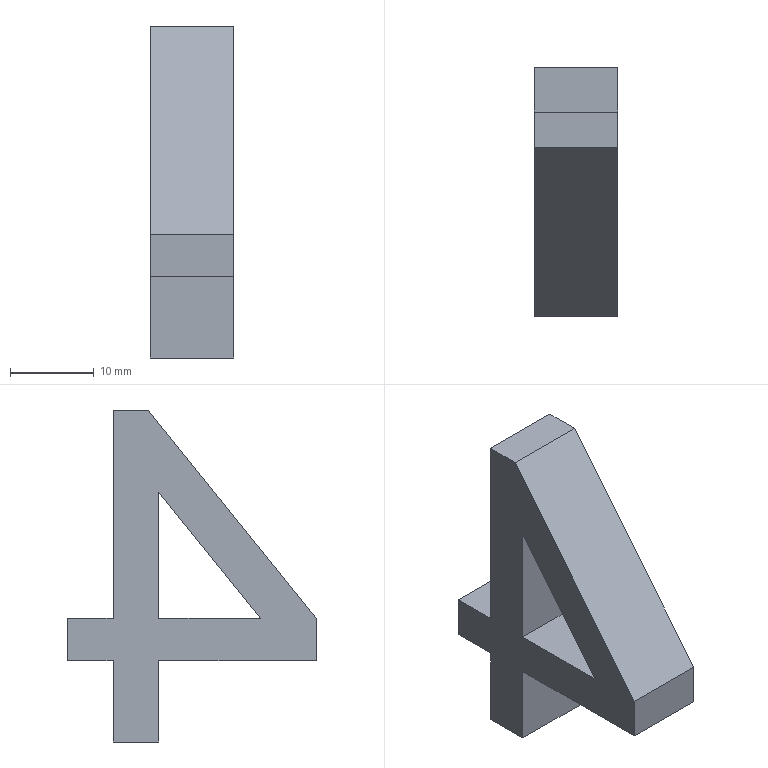Part | NX | features solid 2 | 1 solid | 16 faces | box 10 x 29.69 x 39.602 mm | volume 4649 mm3 | plane 16
STEP:
#1=CARTESIAN_POINT('',(2250.,-423.385,-655.254));
#2=VERTEX_POINT('',#1);
#3=CARTESIAN_POINT('',(2250.,-423.385,-640.218));
#4=VERTEX_POINT('',#3);
#5=CARTESIAN_POINT('',(2250.,-423.385,-655.254));
#6=CARTESIAN_POINT('',(2250.,-423.385,-650.242));
#7=CARTESIAN_POINT('',(2250.,-423.385,-645.23));
#8=CARTESIAN_POINT('',(2250.,-423.385,-640.218));
#9=B_SPLINE_CURVE_WITH_KNOTS('',3,(#5,#6,#7,#8),.UNSPECIFIED.,.F.,.F.,(4,4),(0.2613,0.5844),.PIECEWISE_BEZIER_KNOTS.);
#10=EDGE_CURVE('',#2,#4,#9,.T.);
#11=ORIENTED_EDGE('',*,*,#10,.F.);
#12=CARTESIAN_POINT('',(2260.,-423.385,-655.254));
#13=VERTEX_POINT('',#12);
#14=CARTESIAN_POINT('',(2260.,-423.385,-655.254));
#15=DIRECTION('',(-1.,0.,0.));
#16=VECTOR('',#15,1000.);
#17=LINE('',#14,#16);
#18=EDGE_CURVE('',#13,#2,#17,.T.);
#19=ORIENTED_EDGE('',*,*,#18,.F.);
#20=CARTESIAN_POINT('',(2260.,-423.385,-640.218));
#21=VERTEX_POINT('',#20);
#22=CARTESIAN_POINT('',(2260.,-423.385,-655.254));
#23=CARTESIAN_POINT('',(2260.,-423.385,-650.242));
#24=CARTESIAN_POINT('',(2260.,-423.385,-645.23));
#25=CARTESIAN_POINT('',(2260.,-423.385,-640.218));
#26=B_SPLINE_CURVE_WITH_KNOTS('',3,(#22,#23,#24,#25),.UNSPECIFIED.,.F.,.F.,(4,4),(0.2613,0.5844),.PIECEWISE_BEZIER_KNOTS.);
#27=EDGE_CURVE('',#13,#21,#26,.T.);
#28=ORIENTED_EDGE('',*,*,#27,.T.);
#29=CARTESIAN_POINT('',(2260.,-423.385,-640.218));
#30=DIRECTION('',(-1.,0.,0.));
#31=VECTOR('',#30,1000.);
#32=LINE('',#29,#31);
#33=EDGE_CURVE('',#21,#4,#32,.T.);
#34=ORIENTED_EDGE('',*,*,#33,.T.);
#35=EDGE_LOOP('',(#11,#19,#28,#34));
#36=FACE_BOUND('',#35,.T.);
#37=CARTESIAN_POINT('',(2260.,-423.385,-655.254));
#38=DIRECTION('',(0.,-1.,0.));
#39=DIRECTION('',(1.,0.,0.));
#40=AXIS2_PLACEMENT_3D('',#37,#38,#39);
#41=PLANE('',#40);
#42=ADVANCED_FACE('',(#36),#41,.T.);
#43=CARTESIAN_POINT('',(2250.,-435.546,-655.254));
#44=VERTEX_POINT('',#43);
#45=CARTESIAN_POINT('',(2250.,-423.385,-640.218));
#46=CARTESIAN_POINT('',(2250.,-427.439,-645.23));
#47=CARTESIAN_POINT('',(2250.,-431.493,-650.242));
#48=CARTESIAN_POINT('',(2250.,-435.546,-655.254));
#49=B_SPLINE_CURVE_WITH_KNOTS('',3,(#45,#46,#47,#48),.UNSPECIFIED.,.F.,.F.,(4,4),(0.5844,1.),.PIECEWISE_BEZIER_KNOTS.);
#50=EDGE_CURVE('',#4,#44,#49,.T.);
#51=ORIENTED_EDGE('',*,*,#50,.F.);
#52=ORIENTED_EDGE('',*,*,#33,.F.);
#53=CARTESIAN_POINT('',(2260.,-435.546,-655.254));
#54=VERTEX_POINT('',#53);
#55=CARTESIAN_POINT('',(2260.,-423.385,-640.218));
#56=CARTESIAN_POINT('',(2260.,-427.439,-645.23));
#57=CARTESIAN_POINT('',(2260.,-431.493,-650.242));
#58=CARTESIAN_POINT('',(2260.,-435.546,-655.254));
#59=B_SPLINE_CURVE_WITH_KNOTS('',3,(#55,#56,#57,#58),.UNSPECIFIED.,.F.,.F.,(4,4),(0.5844,1.),.PIECEWISE_BEZIER_KNOTS.);
#60=EDGE_CURVE('',#21,#54,#59,.T.);
#61=ORIENTED_EDGE('',*,*,#60,.T.);
#62=CARTESIAN_POINT('',(2260.,-435.546,-655.254));
#63=DIRECTION('',(-1.,0.,0.));
#64=VECTOR('',#63,1000.);
#65=LINE('',#62,#64);
#66=EDGE_CURVE('',#54,#44,#65,.T.);
#67=ORIENTED_EDGE('',*,*,#66,.T.);
#68=EDGE_LOOP('',(#51,#52,#61,#67));
#69=FACE_BOUND('',#68,.T.);
#70=CARTESIAN_POINT('',(2260.,-423.385,-640.218));
#71=DIRECTION('',(0.,0.7775,-0.6288));
#72=DIRECTION('',(0.,0.6288,0.7775));
#73=AXIS2_PLACEMENT_3D('',#70,#71,#72);
#74=PLANE('',#73);
#75=ADVANCED_FACE('',(#69),#74,.T.);
#76=CARTESIAN_POINT('',(2250.,-417.94,-670.));
#77=VERTEX_POINT('',#76);
#78=CARTESIAN_POINT('',(2250.,-423.385,-670.));
#79=VERTEX_POINT('',#78);
#80=CARTESIAN_POINT('',(2250.,-417.94,-670.));
#81=CARTESIAN_POINT('',(2250.,-419.755,-670.));
#82=CARTESIAN_POINT('',(2250.,-421.57,-670.));
#83=CARTESIAN_POINT('',(2250.,-423.385,-670.));
#84=B_SPLINE_CURVE_WITH_KNOTS('',3,(#80,#81,#82,#83),.UNSPECIFIED.,.F.,.F.,(4,4),(0.,0.04335),.PIECEWISE_BEZIER_KNOTS.);
#85=EDGE_CURVE('',#77,#79,#84,.T.);
#86=ORIENTED_EDGE('',*,*,#85,.F.);
#87=CARTESIAN_POINT('',(2260.,-417.94,-670.));
#88=VERTEX_POINT('',#87);
#89=CARTESIAN_POINT('',(2260.,-417.94,-670.));
#90=DIRECTION('',(-1.,0.,0.));
#91=VECTOR('',#90,1000.);
#92=LINE('',#89,#91);
#93=EDGE_CURVE('',#88,#77,#92,.T.);
#94=ORIENTED_EDGE('',*,*,#93,.F.);
#95=CARTESIAN_POINT('',(2260.,-423.385,-670.));
#96=VERTEX_POINT('',#95);
#97=CARTESIAN_POINT('',(2260.,-417.94,-670.));
#98=CARTESIAN_POINT('',(2260.,-419.755,-670.));
#99=CARTESIAN_POINT('',(2260.,-421.57,-670.));
#100=CARTESIAN_POINT('',(2260.,-423.385,-670.));
#101=B_SPLINE_CURVE_WITH_KNOTS('',3,(#97,#98,#99,#100),.UNSPECIFIED.,.F.,.F.,(4,4),(0.,0.04335),.PIECEWISE_BEZIER_KNOTS.);
#102=EDGE_CURVE('',#88,#96,#101,.T.);
#103=ORIENTED_EDGE('',*,*,#102,.T.);
#104=CARTESIAN_POINT('',(2260.,-423.385,-670.));
#105=DIRECTION('',(-1.,0.,0.));
#106=VECTOR('',#105,1000.);
#107=LINE('',#104,#106);
#108=EDGE_CURVE('',#96,#79,#107,.T.);
#109=ORIENTED_EDGE('',*,*,#108,.T.);
#110=EDGE_LOOP('',(#86,#94,#103,#109));
#111=FACE_BOUND('',#110,.T.);
#112=CARTESIAN_POINT('',(2260.,-417.94,-670.));
#113=DIRECTION('',(0.,0.,-1.));
#114=DIRECTION('',(-1.,0.,0.));
#115=AXIS2_PLACEMENT_3D('',#112,#113,#114);
#116=PLANE('',#115);
#117=ADVANCED_FACE('',(#111),#116,.T.);
#118=CARTESIAN_POINT('',(2250.,-423.385,-660.302));
#119=VERTEX_POINT('',#118);
#120=CARTESIAN_POINT('',(2250.,-423.385,-670.));
#121=CARTESIAN_POINT('',(2250.,-423.385,-666.767));
#122=CARTESIAN_POINT('',(2250.,-423.385,-663.535));
#123=CARTESIAN_POINT('',(2250.,-423.385,-660.302));
#124=B_SPLINE_CURVE_WITH_KNOTS('',3,(#120,#121,#122,#123),.UNSPECIFIED.,.F.,.F.,(4,4),(0.04335,0.1206),.PIECEWISE_BEZIER_KNOTS.);
#125=EDGE_CURVE('',#79,#119,#124,.T.);
#126=ORIENTED_EDGE('',*,*,#125,.F.);
#127=ORIENTED_EDGE('',*,*,#108,.F.);
#128=CARTESIAN_POINT('',(2260.,-423.385,-660.302));
#129=VERTEX_POINT('',#128);
#130=CARTESIAN_POINT('',(2260.,-423.385,-670.));
#131=CARTESIAN_POINT('',(2260.,-423.385,-666.767));
#132=CARTESIAN_POINT('',(2260.,-423.385,-663.535));
#133=CARTESIAN_POINT('',(2260.,-423.385,-660.302));
#134=B_SPLINE_CURVE_WITH_KNOTS('',3,(#130,#131,#132,#133),.UNSPECIFIED.,.F.,.F.,(4,4),(0.04335,0.1206),.PIECEWISE_BEZIER_KNOTS.);
#135=EDGE_CURVE('',#96,#129,#134,.T.);
#136=ORIENTED_EDGE('',*,*,#135,.T.);
#137=CARTESIAN_POINT('',(2260.,-423.385,-660.302));
#138=DIRECTION('',(-1.,0.,0.));
#139=VECTOR('',#138,1000.);
#140=LINE('',#137,#139);
#141=EDGE_CURVE('',#129,#119,#140,.T.);
#142=ORIENTED_EDGE('',*,*,#141,.T.);
#143=EDGE_LOOP('',(#126,#127,#136,#142));
#144=FACE_BOUND('',#143,.T.);
#145=CARTESIAN_POINT('',(2260.,-423.385,-670.));
#146=DIRECTION('',(0.,-1.,0.));
#147=DIRECTION('',(1.,0.,0.));
#148=AXIS2_PLACEMENT_3D('',#145,#146,#147);
#149=PLANE('',#148);
#150=ADVANCED_FACE('',(#144),#149,.T.);
#151=CARTESIAN_POINT('',(2250.,-442.2,-660.302));
#152=VERTEX_POINT('',#151);
#153=CARTESIAN_POINT('',(2250.,-423.385,-660.302));
#154=CARTESIAN_POINT('',(2250.,-429.657,-660.302));
#155=CARTESIAN_POINT('',(2250.,-435.928,-660.302));
#156=CARTESIAN_POINT('',(2250.,-442.2,-660.302));
#157=B_SPLINE_CURVE_WITH_KNOTS('',3,(#153,#154,#155,#156),.UNSPECIFIED.,.F.,.F.,(4,4),(0.1206,0.2704),.PIECEWISE_BEZIER_KNOTS.);
#158=EDGE_CURVE('',#119,#152,#157,.T.);
#159=ORIENTED_EDGE('',*,*,#158,.F.);
#160=ORIENTED_EDGE('',*,*,#141,.F.);
#161=CARTESIAN_POINT('',(2260.,-442.2,-660.302));
#162=VERTEX_POINT('',#161);
#163=CARTESIAN_POINT('',(2260.,-423.385,-660.302));
#164=CARTESIAN_POINT('',(2260.,-429.657,-660.302));
#165=CARTESIAN_POINT('',(2260.,-435.928,-660.302));
#166=CARTESIAN_POINT('',(2260.,-442.2,-660.302));
#167=B_SPLINE_CURVE_WITH_KNOTS('',3,(#163,#164,#165,#166),.UNSPECIFIED.,.F.,.F.,(4,4),(0.1206,0.2704),.PIECEWISE_BEZIER_KNOTS.);
#168=EDGE_CURVE('',#129,#162,#167,.T.);
#169=ORIENTED_EDGE('',*,*,#168,.T.);
#170=CARTESIAN_POINT('',(2260.,-442.2,-660.302));
#171=DIRECTION('',(-1.,0.,0.));
#172=VECTOR('',#171,1000.);
#173=LINE('',#170,#172);
#174=EDGE_CURVE('',#162,#152,#173,.T.);
#175=ORIENTED_EDGE('',*,*,#174,.T.);
#176=EDGE_LOOP('',(#159,#160,#169,#175));
#177=FACE_BOUND('',#176,.T.);
#178=CARTESIAN_POINT('',(2260.,-423.385,-660.302));
#179=DIRECTION('',(0.,0.,-1.));
#180=DIRECTION('',(-1.,0.,0.));
#181=AXIS2_PLACEMENT_3D('',#178,#179,#180);
#182=PLANE('',#181);
#183=ADVANCED_FACE('',(#177),#182,.T.);
#184=CARTESIAN_POINT('',(2250.,-442.2,-655.254));
#185=VERTEX_POINT('',#184);
#186=CARTESIAN_POINT('',(2250.,-442.2,-660.302));
#187=CARTESIAN_POINT('',(2250.,-442.2,-658.62));
#188=CARTESIAN_POINT('',(2250.,-442.2,-656.937));
#189=CARTESIAN_POINT('',(2250.,-442.2,-655.254));
#190=B_SPLINE_CURVE_WITH_KNOTS('',3,(#186,#187,#188,#189),.UNSPECIFIED.,.F.,.F.,(4,4),(0.2704,0.3105),.PIECEWISE_BEZIER_KNOTS.);
#191=EDGE_CURVE('',#152,#185,#190,.T.);
#192=ORIENTED_EDGE('',*,*,#191,.F.);
#193=ORIENTED_EDGE('',*,*,#174,.F.);
#194=CARTESIAN_POINT('',(2260.,-442.2,-655.254));
#195=VERTEX_POINT('',#194);
#196=CARTESIAN_POINT('',(2260.,-442.2,-660.302));
#197=CARTESIAN_POINT('',(2260.,-442.2,-658.62));
#198=CARTESIAN_POINT('',(2260.,-442.2,-656.937));
#199=CARTESIAN_POINT('',(2260.,-442.2,-655.254));
#200=B_SPLINE_CURVE_WITH_KNOTS('',3,(#196,#197,#198,#199),.UNSPECIFIED.,.F.,.F.,(4,4),(0.2704,0.3105),.PIECEWISE_BEZIER_KNOTS.);
#201=EDGE_CURVE('',#162,#195,#200,.T.);
#202=ORIENTED_EDGE('',*,*,#201,.T.);
#203=CARTESIAN_POINT('',(2260.,-442.2,-655.254));
#204=DIRECTION('',(-1.,0.,0.));
#205=VECTOR('',#204,1000.);
#206=LINE('',#203,#205);
#207=EDGE_CURVE('',#195,#185,#206,.T.);
#208=ORIENTED_EDGE('',*,*,#207,.T.);
#209=EDGE_LOOP('',(#192,#193,#202,#208));
#210=FACE_BOUND('',#209,.T.);
#211=CARTESIAN_POINT('',(2260.,-442.2,-660.302));
#212=DIRECTION('',(0.,-1.,0.));
#213=DIRECTION('',(1.,0.,0.));
#214=AXIS2_PLACEMENT_3D('',#211,#212,#213);
#215=PLANE('',#214);
#216=ADVANCED_FACE('',(#210),#215,.T.);
#217=CARTESIAN_POINT('',(2250.,-422.131,-630.398));
#218=VERTEX_POINT('',#217);
#219=CARTESIAN_POINT('',(2250.,-442.2,-655.254));
#220=CARTESIAN_POINT('',(2250.,-435.51,-646.969));
#221=CARTESIAN_POINT('',(2250.,-428.821,-638.683));
#222=CARTESIAN_POINT('',(2250.,-422.131,-630.398));
#223=B_SPLINE_CURVE_WITH_KNOTS('',3,(#219,#220,#221,#222),.UNSPECIFIED.,.F.,.F.,(4,4),(0.3105,0.5649),.PIECEWISE_BEZIER_KNOTS.);
#224=EDGE_CURVE('',#185,#218,#223,.T.);
#225=ORIENTED_EDGE('',*,*,#224,.F.);
#226=ORIENTED_EDGE('',*,*,#207,.F.);
#227=CARTESIAN_POINT('',(2260.,-422.131,-630.398));
#228=VERTEX_POINT('',#227);
#229=CARTESIAN_POINT('',(2260.,-442.2,-655.254));
#230=CARTESIAN_POINT('',(2260.,-435.51,-646.969));
#231=CARTESIAN_POINT('',(2260.,-428.821,-638.683));
#232=CARTESIAN_POINT('',(2260.,-422.131,-630.398));
#233=B_SPLINE_CURVE_WITH_KNOTS('',3,(#229,#230,#231,#232),.UNSPECIFIED.,.F.,.F.,(4,4),(0.3105,0.5649),.PIECEWISE_BEZIER_KNOTS.);
#234=EDGE_CURVE('',#195,#228,#233,.T.);
#235=ORIENTED_EDGE('',*,*,#234,.T.);
#236=CARTESIAN_POINT('',(2260.,-422.131,-630.398));
#237=DIRECTION('',(-1.,0.,0.));
#238=VECTOR('',#237,1000.);
#239=LINE('',#236,#238);
#240=EDGE_CURVE('',#228,#218,#239,.T.);
#241=ORIENTED_EDGE('',*,*,#240,.T.);
#242=EDGE_LOOP('',(#225,#226,#235,#241));
#243=FACE_BOUND('',#242,.T.);
#244=CARTESIAN_POINT('',(2260.,-442.2,-655.254));
#245=DIRECTION('',(0.,-0.7781,0.6282));
#246=DIRECTION('',(0.,-0.6282,-0.7781));
#247=AXIS2_PLACEMENT_3D('',#244,#245,#246);
#248=PLANE('',#247);
#249=ADVANCED_FACE('',(#243),#248,.T.);
#250=CARTESIAN_POINT('',(2250.,-417.94,-630.398));
#251=VERTEX_POINT('',#250);
#252=CARTESIAN_POINT('',(2250.,-422.131,-630.398));
#253=CARTESIAN_POINT('',(2250.,-420.734,-630.398));
#254=CARTESIAN_POINT('',(2250.,-419.337,-630.398));
#255=CARTESIAN_POINT('',(2250.,-417.94,-630.398));
#256=B_SPLINE_CURVE_WITH_KNOTS('',3,(#252,#253,#254,#255),.UNSPECIFIED.,.F.,.F.,(4,4),(0.5649,0.5982),.PIECEWISE_BEZIER_KNOTS.);
#257=EDGE_CURVE('',#218,#251,#256,.T.);
#258=ORIENTED_EDGE('',*,*,#257,.F.);
#259=ORIENTED_EDGE('',*,*,#240,.F.);
#260=CARTESIAN_POINT('',(2260.,-417.94,-630.398));
#261=VERTEX_POINT('',#260);
#262=CARTESIAN_POINT('',(2260.,-422.131,-630.398));
#263=CARTESIAN_POINT('',(2260.,-420.734,-630.398));
#264=CARTESIAN_POINT('',(2260.,-419.337,-630.398));
#265=CARTESIAN_POINT('',(2260.,-417.94,-630.398));
#266=B_SPLINE_CURVE_WITH_KNOTS('',3,(#262,#263,#264,#265),.UNSPECIFIED.,.F.,.F.,(4,4),(0.5649,0.5982),.PIECEWISE_BEZIER_KNOTS.);
#267=EDGE_CURVE('',#228,#261,#266,.T.);
#268=ORIENTED_EDGE('',*,*,#267,.T.);
#269=CARTESIAN_POINT('',(2260.,-417.94,-630.398));
#270=DIRECTION('',(-1.,0.,0.));
#271=VECTOR('',#270,1000.);
#272=LINE('',#269,#271);
#273=EDGE_CURVE('',#261,#251,#272,.T.);
#274=ORIENTED_EDGE('',*,*,#273,.T.);
#275=EDGE_LOOP('',(#258,#259,#268,#274));
#276=FACE_BOUND('',#275,.T.);
#277=CARTESIAN_POINT('',(2260.,-422.131,-630.398));
#278=DIRECTION('',(0.,0.,1.));
#279=DIRECTION('',(1.,0.,0.));
#280=AXIS2_PLACEMENT_3D('',#277,#278,#279);
#281=PLANE('',#280);
#282=ADVANCED_FACE('',(#276),#281,.T.);
#283=CARTESIAN_POINT('',(2250.,-417.94,-655.254));
#284=VERTEX_POINT('',#283);
#285=CARTESIAN_POINT('',(2250.,-417.94,-630.398));
#286=CARTESIAN_POINT('',(2250.,-417.94,-638.683));
#287=CARTESIAN_POINT('',(2250.,-417.94,-646.969));
#288=CARTESIAN_POINT('',(2250.,-417.94,-655.254));
#289=B_SPLINE_CURVE_WITH_KNOTS('',3,(#285,#286,#287,#288),.UNSPECIFIED.,.F.,.F.,(4,4),(0.5982,0.7961),.PIECEWISE_BEZIER_KNOTS.);
#290=EDGE_CURVE('',#251,#284,#289,.T.);
#291=ORIENTED_EDGE('',*,*,#290,.F.);
#292=ORIENTED_EDGE('',*,*,#273,.F.);
#293=CARTESIAN_POINT('',(2260.,-417.94,-655.254));
#294=VERTEX_POINT('',#293);
#295=CARTESIAN_POINT('',(2260.,-417.94,-630.398));
#296=CARTESIAN_POINT('',(2260.,-417.94,-638.683));
#297=CARTESIAN_POINT('',(2260.,-417.94,-646.969));
#298=CARTESIAN_POINT('',(2260.,-417.94,-655.254));
#299=B_SPLINE_CURVE_WITH_KNOTS('',3,(#295,#296,#297,#298),.UNSPECIFIED.,.F.,.F.,(4,4),(0.5982,0.7961),.PIECEWISE_BEZIER_KNOTS.);
#300=EDGE_CURVE('',#261,#294,#299,.T.);
#301=ORIENTED_EDGE('',*,*,#300,.T.);
#302=CARTESIAN_POINT('',(2260.,-417.94,-655.254));
#303=DIRECTION('',(-1.,0.,0.));
#304=VECTOR('',#303,1000.);
#305=LINE('',#302,#304);
#306=EDGE_CURVE('',#294,#284,#305,.T.);
#307=ORIENTED_EDGE('',*,*,#306,.T.);
#308=EDGE_LOOP('',(#291,#292,#301,#307));
#309=FACE_BOUND('',#308,.T.);
#310=CARTESIAN_POINT('',(2260.,-417.94,-630.398));
#311=DIRECTION('',(0.,1.,0.));
#312=DIRECTION('',(-1.,0.,0.));
#313=AXIS2_PLACEMENT_3D('',#310,#311,#312);
#314=PLANE('',#313);
#315=ADVANCED_FACE('',(#309),#314,.T.);
#316=CARTESIAN_POINT('',(2250.,-412.51,-655.254));
#317=VERTEX_POINT('',#316);
#318=CARTESIAN_POINT('',(2250.,-417.94,-655.254));
#319=CARTESIAN_POINT('',(2250.,-416.13,-655.254));
#320=CARTESIAN_POINT('',(2250.,-414.32,-655.254));
#321=CARTESIAN_POINT('',(2250.,-412.51,-655.254));
#322=B_SPLINE_CURVE_WITH_KNOTS('',3,(#318,#319,#320,#321),.UNSPECIFIED.,.F.,.F.,(4,4),(0.7961,0.8394),.PIECEWISE_BEZIER_KNOTS.);
#323=EDGE_CURVE('',#284,#317,#322,.T.);
#324=ORIENTED_EDGE('',*,*,#323,.F.);
#325=ORIENTED_EDGE('',*,*,#306,.F.);
#326=CARTESIAN_POINT('',(2260.,-412.51,-655.254));
#327=VERTEX_POINT('',#326);
#328=CARTESIAN_POINT('',(2260.,-417.94,-655.254));
#329=CARTESIAN_POINT('',(2260.,-416.13,-655.254));
#330=CARTESIAN_POINT('',(2260.,-414.32,-655.254));
#331=CARTESIAN_POINT('',(2260.,-412.51,-655.254));
#332=B_SPLINE_CURVE_WITH_KNOTS('',3,(#328,#329,#330,#331),.UNSPECIFIED.,.F.,.F.,(4,4),(0.7961,0.8394),.PIECEWISE_BEZIER_KNOTS.);
#333=EDGE_CURVE('',#294,#327,#332,.T.);
#334=ORIENTED_EDGE('',*,*,#333,.T.);
#335=CARTESIAN_POINT('',(2260.,-412.51,-655.254));
#336=DIRECTION('',(-1.,0.,0.));
#337=VECTOR('',#336,1000.);
#338=LINE('',#335,#337);
#339=EDGE_CURVE('',#327,#317,#338,.T.);
#340=ORIENTED_EDGE('',*,*,#339,.T.);
#341=EDGE_LOOP('',(#324,#325,#334,#340));
#342=FACE_BOUND('',#341,.T.);
#343=CARTESIAN_POINT('',(2260.,-417.94,-655.254));
#344=DIRECTION('',(0.,0.,1.));
#345=DIRECTION('',(1.,0.,0.));
#346=AXIS2_PLACEMENT_3D('',#343,#344,#345);
#347=PLANE('',#346);
#348=ADVANCED_FACE('',(#342),#347,.T.);
#349=CARTESIAN_POINT('',(2250.,-412.51,-660.302));
#350=VERTEX_POINT('',#349);
#351=CARTESIAN_POINT('',(2250.,-412.51,-655.254));
#352=CARTESIAN_POINT('',(2250.,-412.51,-656.937));
#353=CARTESIAN_POINT('',(2250.,-412.51,-658.62));
#354=CARTESIAN_POINT('',(2250.,-412.51,-660.302));
#355=B_SPLINE_CURVE_WITH_KNOTS('',3,(#351,#352,#353,#354),.UNSPECIFIED.,.F.,.F.,(4,4),(0.8394,0.8796),.PIECEWISE_BEZIER_KNOTS.);
#356=EDGE_CURVE('',#317,#350,#355,.T.);
#357=ORIENTED_EDGE('',*,*,#356,.F.);
#358=ORIENTED_EDGE('',*,*,#339,.F.);
#359=CARTESIAN_POINT('',(2260.,-412.51,-660.302));
#360=VERTEX_POINT('',#359);
#361=CARTESIAN_POINT('',(2260.,-412.51,-655.254));
#362=CARTESIAN_POINT('',(2260.,-412.51,-656.937));
#363=CARTESIAN_POINT('',(2260.,-412.51,-658.62));
#364=CARTESIAN_POINT('',(2260.,-412.51,-660.302));
#365=B_SPLINE_CURVE_WITH_KNOTS('',3,(#361,#362,#363,#364),.UNSPECIFIED.,.F.,.F.,(4,4),(0.8394,0.8796),.PIECEWISE_BEZIER_KNOTS.);
#366=EDGE_CURVE('',#327,#360,#365,.T.);
#367=ORIENTED_EDGE('',*,*,#366,.T.);
#368=CARTESIAN_POINT('',(2260.,-412.51,-660.302));
#369=DIRECTION('',(-1.,0.,0.));
#370=VECTOR('',#369,1000.);
#371=LINE('',#368,#370);
#372=EDGE_CURVE('',#360,#350,#371,.T.);
#373=ORIENTED_EDGE('',*,*,#372,.T.);
#374=EDGE_LOOP('',(#357,#358,#367,#373));
#375=FACE_BOUND('',#374,.T.);
#376=CARTESIAN_POINT('',(2260.,-412.51,-655.254));
#377=DIRECTION('',(0.,1.,0.));
#378=DIRECTION('',(-1.,0.,0.));
#379=AXIS2_PLACEMENT_3D('',#376,#377,#378);
#380=PLANE('',#379);
#381=ADVANCED_FACE('',(#375),#380,.T.);
#382=CARTESIAN_POINT('',(2250.,-417.94,-660.302));
#383=VERTEX_POINT('',#382);
#384=CARTESIAN_POINT('',(2250.,-412.51,-660.302));
#385=CARTESIAN_POINT('',(2250.,-414.32,-660.302));
#386=CARTESIAN_POINT('',(2250.,-416.13,-660.302));
#387=CARTESIAN_POINT('',(2250.,-417.94,-660.302));
#388=B_SPLINE_CURVE_WITH_KNOTS('',3,(#384,#385,#386,#387),.UNSPECIFIED.,.F.,.F.,(4,4),(0.8796,0.9228),.PIECEWISE_BEZIER_KNOTS.);
#389=EDGE_CURVE('',#350,#383,#388,.T.);
#390=ORIENTED_EDGE('',*,*,#389,.F.);
#391=ORIENTED_EDGE('',*,*,#372,.F.);
#392=CARTESIAN_POINT('',(2260.,-417.94,-660.302));
#393=VERTEX_POINT('',#392);
#394=CARTESIAN_POINT('',(2260.,-412.51,-660.302));
#395=CARTESIAN_POINT('',(2260.,-414.32,-660.302));
#396=CARTESIAN_POINT('',(2260.,-416.13,-660.302));
#397=CARTESIAN_POINT('',(2260.,-417.94,-660.302));
#398=B_SPLINE_CURVE_WITH_KNOTS('',3,(#394,#395,#396,#397),.UNSPECIFIED.,.F.,.F.,(4,4),(0.8796,0.9228),.PIECEWISE_BEZIER_KNOTS.);
#399=EDGE_CURVE('',#360,#393,#398,.T.);
#400=ORIENTED_EDGE('',*,*,#399,.T.);
#401=CARTESIAN_POINT('',(2260.,-417.94,-660.302));
#402=DIRECTION('',(-1.,0.,0.));
#403=VECTOR('',#402,1000.);
#404=LINE('',#401,#403);
#405=EDGE_CURVE('',#393,#383,#404,.T.);
#406=ORIENTED_EDGE('',*,*,#405,.T.);
#407=EDGE_LOOP('',(#390,#391,#400,#406));
#408=FACE_BOUND('',#407,.T.);
#409=CARTESIAN_POINT('',(2260.,-412.51,-660.302));
#410=DIRECTION('',(0.,0.,-1.));
#411=DIRECTION('',(-1.,0.,0.));
#412=AXIS2_PLACEMENT_3D('',#409,#410,#411);
#413=PLANE('',#412);
#414=ADVANCED_FACE('',(#408),#413,.T.);
#415=CARTESIAN_POINT('',(2250.,-417.94,-660.302));
#416=CARTESIAN_POINT('',(2250.,-417.94,-663.535));
#417=CARTESIAN_POINT('',(2250.,-417.94,-666.767));
#418=CARTESIAN_POINT('',(2250.,-417.94,-670.));
#419=B_SPLINE_CURVE_WITH_KNOTS('',3,(#415,#416,#417,#418),.UNSPECIFIED.,.F.,.F.,(4,4),(0.9228,1.),.PIECEWISE_BEZIER_KNOTS.);
#420=EDGE_CURVE('',#383,#77,#419,.T.);
#421=ORIENTED_EDGE('',*,*,#420,.F.);
#422=ORIENTED_EDGE('',*,*,#405,.F.);
#423=CARTESIAN_POINT('',(2260.,-417.94,-660.302));
#424=CARTESIAN_POINT('',(2260.,-417.94,-663.535));
#425=CARTESIAN_POINT('',(2260.,-417.94,-666.767));
#426=CARTESIAN_POINT('',(2260.,-417.94,-670.));
#427=B_SPLINE_CURVE_WITH_KNOTS('',3,(#423,#424,#425,#426),.UNSPECIFIED.,.F.,.F.,(4,4),(0.9228,1.),.PIECEWISE_BEZIER_KNOTS.);
#428=EDGE_CURVE('',#393,#88,#427,.T.);
#429=ORIENTED_EDGE('',*,*,#428,.T.);
#430=ORIENTED_EDGE('',*,*,#93,.T.);
#431=EDGE_LOOP('',(#421,#422,#429,#430));
#432=FACE_BOUND('',#431,.T.);
#433=CARTESIAN_POINT('',(2260.,-417.94,-660.302));
#434=DIRECTION('',(0.,1.,0.));
#435=DIRECTION('',(-1.,0.,0.));
#436=AXIS2_PLACEMENT_3D('',#433,#434,#435);
#437=PLANE('',#436);
#438=ADVANCED_FACE('',(#432),#437,.T.);
#439=CARTESIAN_POINT('',(2250.,-435.546,-655.254));
#440=CARTESIAN_POINT('',(2250.,-431.493,-655.254));
#441=CARTESIAN_POINT('',(2250.,-427.439,-655.254));
#442=CARTESIAN_POINT('',(2250.,-423.385,-655.254));
#443=B_SPLINE_CURVE_WITH_KNOTS('',3,(#439,#440,#441,#442),.UNSPECIFIED.,.F.,.F.,(4,4),(0.,0.2613),.PIECEWISE_BEZIER_KNOTS.);
#444=EDGE_CURVE('',#44,#2,#443,.T.);
#445=ORIENTED_EDGE('',*,*,#444,.F.);
#446=ORIENTED_EDGE('',*,*,#66,.F.);
#447=CARTESIAN_POINT('',(2260.,-435.546,-655.254));
#448=CARTESIAN_POINT('',(2260.,-431.493,-655.254));
#449=CARTESIAN_POINT('',(2260.,-427.439,-655.254));
#450=CARTESIAN_POINT('',(2260.,-423.385,-655.254));
#451=B_SPLINE_CURVE_WITH_KNOTS('',3,(#447,#448,#449,#450),.UNSPECIFIED.,.F.,.F.,(4,4),(0.,0.2613),.PIECEWISE_BEZIER_KNOTS.);
#452=EDGE_CURVE('',#54,#13,#451,.T.);
#453=ORIENTED_EDGE('',*,*,#452,.T.);
#454=ORIENTED_EDGE('',*,*,#18,.T.);
#455=EDGE_LOOP('',(#445,#446,#453,#454));
#456=FACE_BOUND('',#455,.T.);
#457=CARTESIAN_POINT('',(2260.,-435.546,-655.254));
#458=DIRECTION('',(0.,0.,1.));
#459=DIRECTION('',(1.,0.,0.));
#460=AXIS2_PLACEMENT_3D('',#457,#458,#459);
#461=PLANE('',#460);
#462=ADVANCED_FACE('',(#456),#461,.T.);
#463=ORIENTED_EDGE('',*,*,#102,.F.);
#464=ORIENTED_EDGE('',*,*,#428,.F.);
#465=ORIENTED_EDGE('',*,*,#399,.F.);
#466=ORIENTED_EDGE('',*,*,#366,.F.);
#467=ORIENTED_EDGE('',*,*,#333,.F.);
#468=ORIENTED_EDGE('',*,*,#300,.F.);
#469=ORIENTED_EDGE('',*,*,#267,.F.);
#470=ORIENTED_EDGE('',*,*,#234,.F.);
#471=ORIENTED_EDGE('',*,*,#201,.F.);
#472=ORIENTED_EDGE('',*,*,#168,.F.);
#473=ORIENTED_EDGE('',*,*,#135,.F.);
#474=EDGE_LOOP('',(#463,#464,#465,#466,#467,#468,#469,#470,#471,#472,#473));
#475=FACE_BOUND('',#474,.T.);
#476=ORIENTED_EDGE('',*,*,#27,.F.);
#477=ORIENTED_EDGE('',*,*,#452,.F.);
#478=ORIENTED_EDGE('',*,*,#60,.F.);
#479=EDGE_LOOP('',(#476,#477,#478));
#480=FACE_BOUND('',#479,.T.);
#481=CARTESIAN_POINT('',(2260.,-420.663,-670.));
#482=DIRECTION('',(1.,0.,0.));
#483=DIRECTION('',(0.,1.,0.));
#484=AXIS2_PLACEMENT_3D('',#481,#482,#483);
#485=PLANE('',#484);
#486=ADVANCED_FACE('',(#475,#480),#485,.T.);
#487=ORIENTED_EDGE('',*,*,#85,.T.);
#488=ORIENTED_EDGE('',*,*,#125,.T.);
#489=ORIENTED_EDGE('',*,*,#158,.T.);
#490=ORIENTED_EDGE('',*,*,#191,.T.);
#491=ORIENTED_EDGE('',*,*,#224,.T.);
#492=ORIENTED_EDGE('',*,*,#257,.T.);
#493=ORIENTED_EDGE('',*,*,#290,.T.);
#494=ORIENTED_EDGE('',*,*,#323,.T.);
#495=ORIENTED_EDGE('',*,*,#356,.T.);
#496=ORIENTED_EDGE('',*,*,#389,.T.);
#497=ORIENTED_EDGE('',*,*,#420,.T.);
#498=EDGE_LOOP('',(#487,#488,#489,#490,#491,#492,#493,#494,#495,#496,#497));
#499=FACE_BOUND('',#498,.T.);
#500=ORIENTED_EDGE('',*,*,#10,.T.);
#501=ORIENTED_EDGE('',*,*,#50,.T.);
#502=ORIENTED_EDGE('',*,*,#444,.T.);
#503=EDGE_LOOP('',(#500,#501,#502));
#504=FACE_BOUND('',#503,.T.);
#505=CARTESIAN_POINT('',(2250.,-420.663,-670.));
#506=DIRECTION('',(1.,0.,0.));
#507=DIRECTION('',(0.,1.,0.));
#508=AXIS2_PLACEMENT_3D('',#505,#506,#507);
#509=PLANE('',#508);
#510=ADVANCED_FACE('',(#499,#504),#509,.F.);
#511=CLOSED_SHELL('',(#42,#75,#117,#150,#183,#216,#249,#282,#315,#348,#381,#414,#438,#462,#486,#510));
#512=MANIFOLD_SOLID_BREP('',#511);
#513=(LENGTH_UNIT()NAMED_UNIT(*)SI_UNIT(.MILLI.,.METRE.));
#514=UNCERTAINTY_MEASURE_WITH_UNIT(LENGTH_MEASURE(0.00001),#513,'','');
#515=(NAMED_UNIT(*)PLANE_ANGLE_UNIT()SI_UNIT($,.RADIAN.));
#516=(NAMED_UNIT(*)SI_UNIT($,.STERADIAN.)SOLID_ANGLE_UNIT());
#517=(GEOMETRIC_REPRESENTATION_CONTEXT(3)GLOBAL_UNCERTAINTY_ASSIGNED_CONTEXT((#514))GLOBAL_UNIT_ASSIGNED_CONTEXT((#513,#515,#516))REPRESENTATION_CONTEXT('',''));
#518=ADVANCED_BREP_SHAPE_REPRESENTATION('',(#512),#517);